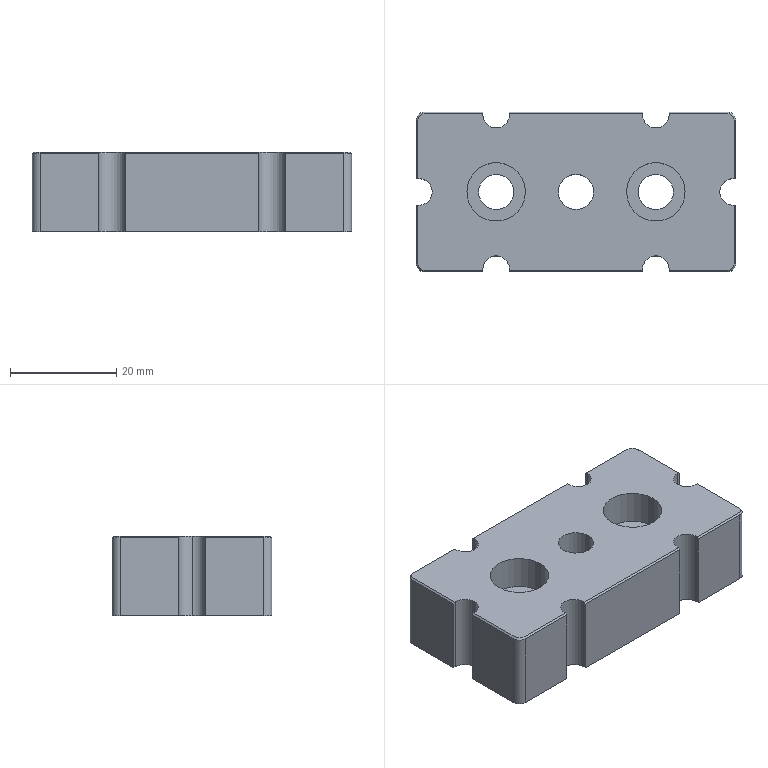Part | STEP file | B2200 end cap_zinc alloy | 1 solid | 61 faces | box 60 x 30 x 15 mm | volume 23538 mm3 | plane 36 | cylinder 21 | cone 4 | commonest cylinder face diameters 5 x7 6.6 x6 3 x4 11 x4